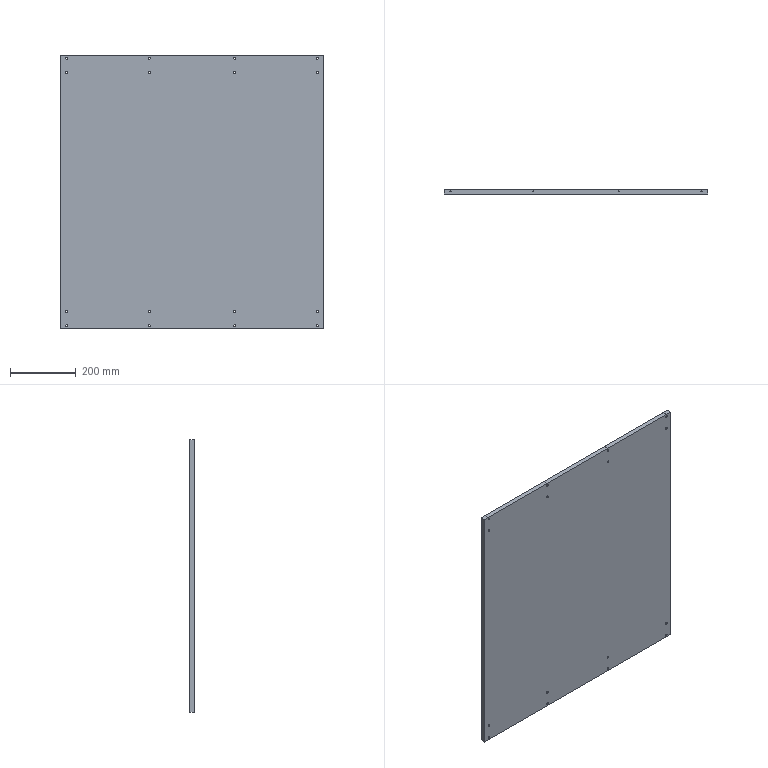Part | STEP file | 0244_207_Plate | 1 solid | 62 faces | box 800 x 15 x 826 mm | volume 9900374 mm3 | cylinder 48 | plane 14 | commonest cylinder face diameters 6.6 x16 6.8 x16 11 x16